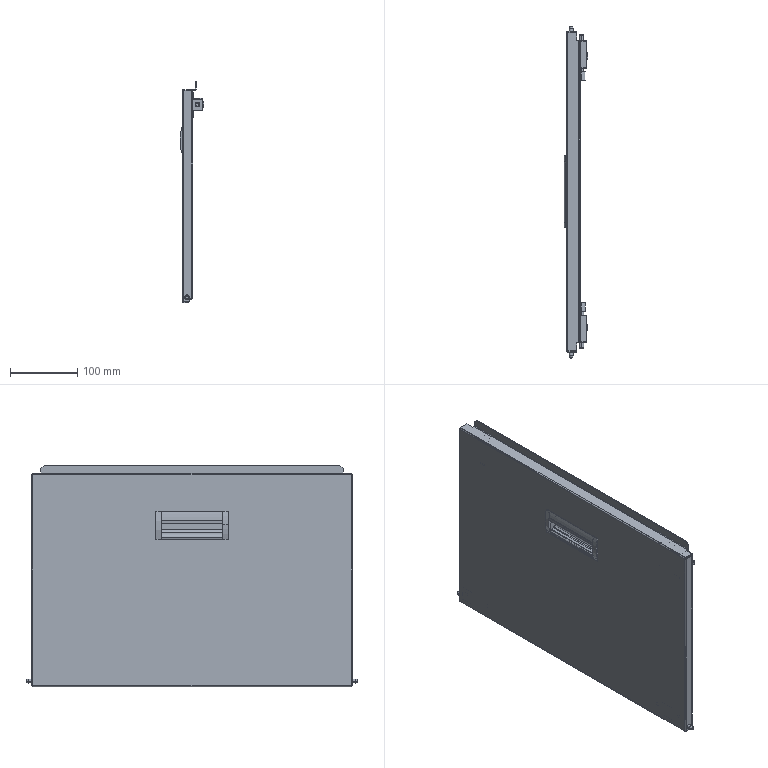Part | SolidWorks | 16 solids | 429 faces | box 35.649 x 494 x 329 mm | volume 327464 mm3 | plane 243 | cylinder 174 | cone 8 | torus 4 | commonest cylinder face diameters 1 x18 2.5 x16 3.2 x16 0.6 x14 7 x13 2 x8